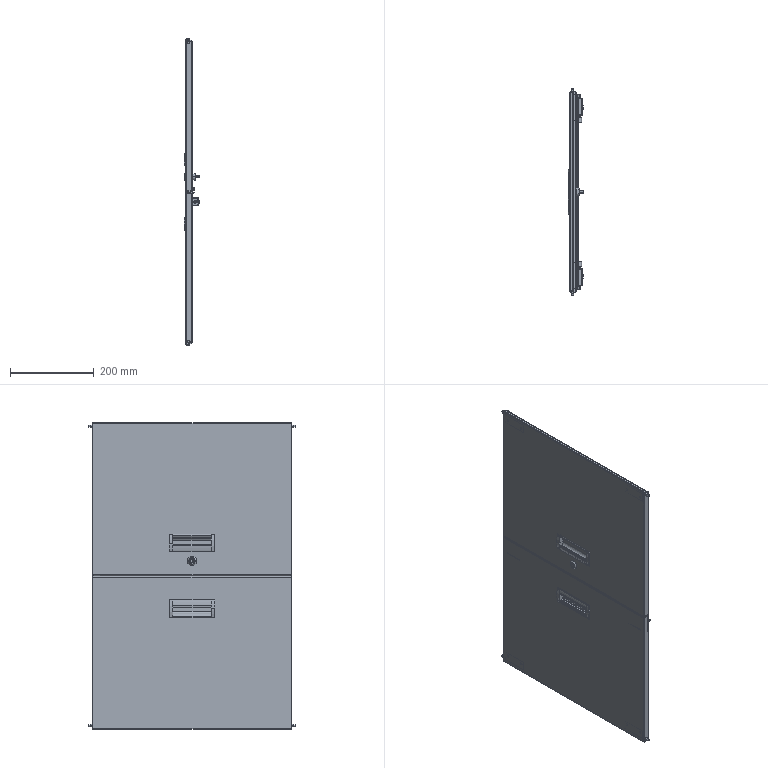Part | SolidWorks | 25 solids | 704 faces | box 37.5 x 494 x 731 mm | volume 708096 mm3 | plane 394 | cylinder 280 | cone 14 | torus 8 | spline 8 | commonest cylinder face diameters 1 x36 7 x23 0.6 x21 2.5 x16 3.2 x16 5.5 x16